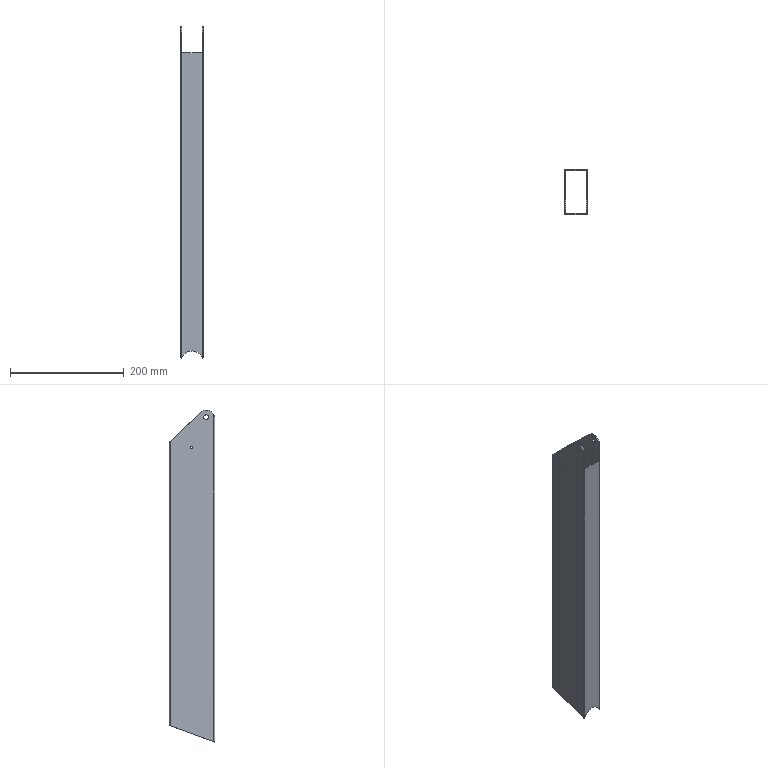Part | STEP file | Q7C0101L | 1 solid | 24 faces | box 40 x 80 x 584.662 mm | volume 247480 mm3 | plane 12 | cylinder 12 | commonest cylinder face diameters 3 x4 3.5 x3 8.5 x2 30 x2 41 x1